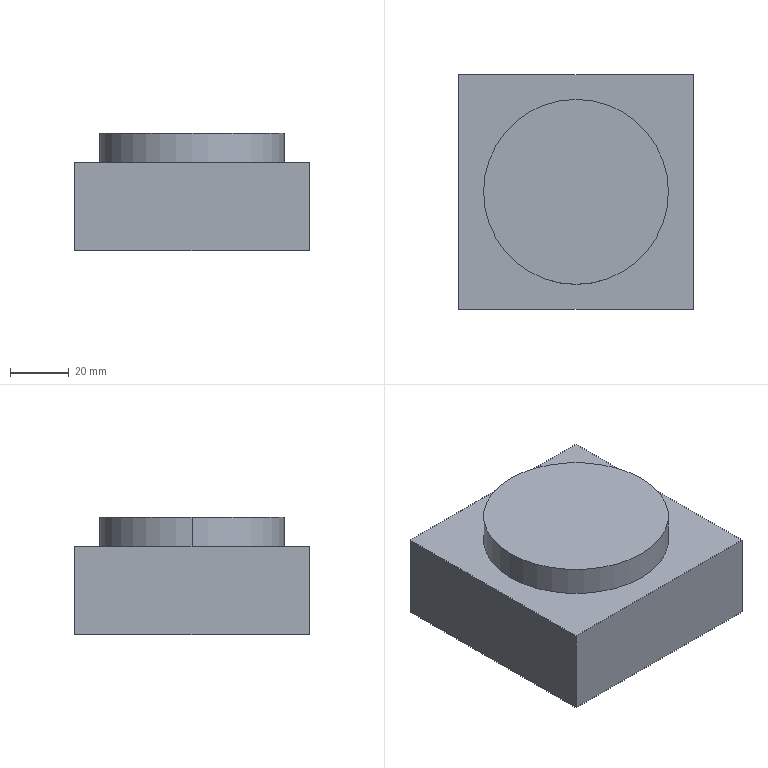Part | SolidWorks | features Extrusion 1, ICE 1 | 1 solid | 9 faces | box 80 x 80 x 40 mm | volume 223172 mm3 | plane 7 | cylinder 2 | commonest cylinder face diameters 63 x2
STEP:
#1=CARTESIAN_POINT('',(31.5,0.,40.));
#2=VERTEX_POINT('',#1);
#3=CARTESIAN_POINT('',(-31.5,0.,40.));
#4=VERTEX_POINT('',#3);
#5=CARTESIAN_POINT('',(0.,0.,40.));
#6=DIRECTION('',(0.,0.,1.));
#7=DIRECTION('',(1.,0.,0.));
#8=AXIS2_PLACEMENT_3D('',#5,#6,#7);
#9=CIRCLE('',#8,31.5);
#10=EDGE_CURVE('',#2,#4,#9,.T.);
#11=ORIENTED_EDGE('',*,*,#10,.F.);
#12=CARTESIAN_POINT('',(31.5,0.,30.));
#13=VERTEX_POINT('',#12);
#14=CARTESIAN_POINT('',(31.5,0.,40.));
#15=DIRECTION('',(0.,0.,-1.));
#16=VECTOR('',#15,1000.);
#17=LINE('',#14,#16);
#18=EDGE_CURVE('',#2,#13,#17,.T.);
#19=ORIENTED_EDGE('',*,*,#18,.T.);
#20=CARTESIAN_POINT('',(-31.5,0.,30.));
#21=VERTEX_POINT('',#20);
#22=CARTESIAN_POINT('',(0.,0.,30.));
#23=DIRECTION('',(0.,0.,1.));
#24=DIRECTION('',(1.,0.,0.));
#25=AXIS2_PLACEMENT_3D('',#22,#23,#24);
#26=CIRCLE('',#25,31.5);
#27=EDGE_CURVE('',#13,#21,#26,.T.);
#28=ORIENTED_EDGE('',*,*,#27,.T.);
#29=CARTESIAN_POINT('',(-31.5,0.,40.));
#30=DIRECTION('',(0.,0.,-1.));
#31=VECTOR('',#30,1000.);
#32=LINE('',#29,#31);
#33=EDGE_CURVE('',#4,#21,#32,.T.);
#34=ORIENTED_EDGE('',*,*,#33,.F.);
#35=EDGE_LOOP('',(#11,#19,#28,#34));
#36=FACE_OUTER_BOUND('',#35,.T.);
#37=CARTESIAN_POINT('',(0.,0.,40.));
#38=DIRECTION('',(0.,0.,-1.));
#39=DIRECTION('',(-1.,0.,0.));
#40=AXIS2_PLACEMENT_3D('',#37,#38,#39);
#41=CYLINDRICAL_SURFACE('',#40,31.5);
#42=ADVANCED_FACE('',(#36),#41,.T.);
#43=CARTESIAN_POINT('',(40.,-40.,0.));
#44=VERTEX_POINT('',#43);
#45=CARTESIAN_POINT('',(40.,40.,0.));
#46=VERTEX_POINT('',#45);
#47=CARTESIAN_POINT('',(40.,-40.,0.));
#48=DIRECTION('',(0.,1.,0.));
#49=VECTOR('',#48,1000.);
#50=LINE('',#47,#49);
#51=EDGE_CURVE('',#44,#46,#50,.T.);
#52=ORIENTED_EDGE('',*,*,#51,.T.);
#53=CARTESIAN_POINT('',(40.,40.,30.));
#54=VERTEX_POINT('',#53);
#55=CARTESIAN_POINT('',(40.,40.,30.));
#56=DIRECTION('',(0.,0.,-1.));
#57=VECTOR('',#56,1000.);
#58=LINE('',#55,#57);
#59=EDGE_CURVE('',#54,#46,#58,.T.);
#60=ORIENTED_EDGE('',*,*,#59,.F.);
#61=CARTESIAN_POINT('',(40.,-40.,30.));
#62=VERTEX_POINT('',#61);
#63=CARTESIAN_POINT('',(40.,-40.,30.));
#64=DIRECTION('',(0.,1.,0.));
#65=VECTOR('',#64,1000.);
#66=LINE('',#63,#65);
#67=EDGE_CURVE('',#62,#54,#66,.T.);
#68=ORIENTED_EDGE('',*,*,#67,.F.);
#69=CARTESIAN_POINT('',(40.,-40.,30.));
#70=DIRECTION('',(0.,0.,-1.));
#71=VECTOR('',#70,1000.);
#72=LINE('',#69,#71);
#73=EDGE_CURVE('',#62,#44,#72,.T.);
#74=ORIENTED_EDGE('',*,*,#73,.T.);
#75=EDGE_LOOP('',(#52,#60,#68,#74));
#76=FACE_OUTER_BOUND('',#75,.T.);
#77=CARTESIAN_POINT('',(40.,-40.,30.));
#78=DIRECTION('',(-1.,0.,0.));
#79=DIRECTION('',(0.,0.,1.));
#80=AXIS2_PLACEMENT_3D('',#77,#78,#79);
#81=PLANE('',#80);
#82=ADVANCED_FACE('',(#76),#81,.F.);
#83=CARTESIAN_POINT('',(-40.,40.,0.));
#84=VERTEX_POINT('',#83);
#85=CARTESIAN_POINT('',(-40.,40.,0.));
#86=DIRECTION('',(-1.,0.,0.));
#87=VECTOR('',#86,1000.);
#88=LINE('',#85,#87);
#89=EDGE_CURVE('',#46,#84,#88,.T.);
#90=ORIENTED_EDGE('',*,*,#89,.T.);
#91=CARTESIAN_POINT('',(-40.,40.,30.));
#92=VERTEX_POINT('',#91);
#93=CARTESIAN_POINT('',(-40.,40.,30.));
#94=DIRECTION('',(0.,0.,-1.));
#95=VECTOR('',#94,1000.);
#96=LINE('',#93,#95);
#97=EDGE_CURVE('',#92,#84,#96,.T.);
#98=ORIENTED_EDGE('',*,*,#97,.F.);
#99=CARTESIAN_POINT('',(-40.,40.,30.));
#100=DIRECTION('',(-1.,0.,0.));
#101=VECTOR('',#100,1000.);
#102=LINE('',#99,#101);
#103=EDGE_CURVE('',#54,#92,#102,.T.);
#104=ORIENTED_EDGE('',*,*,#103,.F.);
#105=ORIENTED_EDGE('',*,*,#59,.T.);
#106=EDGE_LOOP('',(#90,#98,#104,#105));
#107=FACE_OUTER_BOUND('',#106,.T.);
#108=CARTESIAN_POINT('',(-40.,40.,30.));
#109=DIRECTION('',(0.,-1.,0.));
#110=DIRECTION('',(0.,0.,-1.));
#111=AXIS2_PLACEMENT_3D('',#108,#109,#110);
#112=PLANE('',#111);
#113=ADVANCED_FACE('',(#107),#112,.F.);
#114=CARTESIAN_POINT('',(-40.,-40.,0.));
#115=VERTEX_POINT('',#114);
#116=CARTESIAN_POINT('',(-40.,-40.,0.));
#117=DIRECTION('',(0.,-1.,0.));
#118=VECTOR('',#117,1000.);
#119=LINE('',#116,#118);
#120=EDGE_CURVE('',#84,#115,#119,.T.);
#121=ORIENTED_EDGE('',*,*,#120,.T.);
#122=CARTESIAN_POINT('',(-40.,-40.,30.));
#123=VERTEX_POINT('',#122);
#124=CARTESIAN_POINT('',(-40.,-40.,30.));
#125=DIRECTION('',(0.,0.,-1.));
#126=VECTOR('',#125,1000.);
#127=LINE('',#124,#126);
#128=EDGE_CURVE('',#123,#115,#127,.T.);
#129=ORIENTED_EDGE('',*,*,#128,.F.);
#130=CARTESIAN_POINT('',(-40.,-40.,30.));
#131=DIRECTION('',(0.,-1.,0.));
#132=VECTOR('',#131,1000.);
#133=LINE('',#130,#132);
#134=EDGE_CURVE('',#92,#123,#133,.T.);
#135=ORIENTED_EDGE('',*,*,#134,.F.);
#136=ORIENTED_EDGE('',*,*,#97,.T.);
#137=EDGE_LOOP('',(#121,#129,#135,#136));
#138=FACE_OUTER_BOUND('',#137,.T.);
#139=CARTESIAN_POINT('',(-40.,-40.,30.));
#140=DIRECTION('',(1.,0.,0.));
#141=DIRECTION('',(0.,0.,-1.));
#142=AXIS2_PLACEMENT_3D('',#139,#140,#141);
#143=PLANE('',#142);
#144=ADVANCED_FACE('',(#138),#143,.F.);
#145=CARTESIAN_POINT('',(-40.,-40.,0.));
#146=DIRECTION('',(1.,0.,0.));
#147=VECTOR('',#146,1000.);
#148=LINE('',#145,#147);
#149=EDGE_CURVE('',#115,#44,#148,.T.);
#150=ORIENTED_EDGE('',*,*,#149,.T.);
#151=ORIENTED_EDGE('',*,*,#73,.F.);
#152=CARTESIAN_POINT('',(-40.,-40.,30.));
#153=DIRECTION('',(1.,0.,0.));
#154=VECTOR('',#153,1000.);
#155=LINE('',#152,#154);
#156=EDGE_CURVE('',#123,#62,#155,.T.);
#157=ORIENTED_EDGE('',*,*,#156,.F.);
#158=ORIENTED_EDGE('',*,*,#128,.T.);
#159=EDGE_LOOP('',(#150,#151,#157,#158));
#160=FACE_OUTER_BOUND('',#159,.T.);
#161=CARTESIAN_POINT('',(-40.,-40.,30.));
#162=DIRECTION('',(0.,1.,0.));
#163=DIRECTION('',(0.,0.,1.));
#164=AXIS2_PLACEMENT_3D('',#161,#162,#163);
#165=PLANE('',#164);
#166=ADVANCED_FACE('',(#160),#165,.F.);
#167=CARTESIAN_POINT('',(0.,0.,30.));
#168=DIRECTION('',(0.,0.,1.));
#169=DIRECTION('',(1.,0.,0.));
#170=AXIS2_PLACEMENT_3D('',#167,#168,#169);
#171=CIRCLE('',#170,31.5);
#172=EDGE_CURVE('',#21,#13,#171,.T.);
#173=ORIENTED_EDGE('',*,*,#172,.F.);
#174=ORIENTED_EDGE('',*,*,#27,.F.);
#175=EDGE_LOOP('',(#173,#174));
#176=FACE_BOUND('',#175,.T.);
#177=ORIENTED_EDGE('',*,*,#67,.T.);
#178=ORIENTED_EDGE('',*,*,#103,.T.);
#179=ORIENTED_EDGE('',*,*,#134,.T.);
#180=ORIENTED_EDGE('',*,*,#156,.T.);
#181=EDGE_LOOP('',(#177,#178,#179,#180));
#182=FACE_OUTER_BOUND('',#181,.T.);
#183=CARTESIAN_POINT('',(0.,0.,30.));
#184=DIRECTION('',(0.,0.,-1.));
#185=DIRECTION('',(-1.,0.,0.));
#186=AXIS2_PLACEMENT_3D('',#183,#184,#185);
#187=PLANE('',#186);
#188=ADVANCED_FACE('',(#176,#182),#187,.F.);
#189=ORIENTED_EDGE('',*,*,#51,.F.);
#190=ORIENTED_EDGE('',*,*,#149,.F.);
#191=ORIENTED_EDGE('',*,*,#120,.F.);
#192=ORIENTED_EDGE('',*,*,#89,.F.);
#193=EDGE_LOOP('',(#189,#190,#191,#192));
#194=FACE_OUTER_BOUND('',#193,.T.);
#195=CARTESIAN_POINT('',(0.,0.,0.));
#196=DIRECTION('',(0.,0.,-1.));
#197=DIRECTION('',(-1.,0.,0.));
#198=AXIS2_PLACEMENT_3D('',#195,#196,#197);
#199=PLANE('',#198);
#200=ADVANCED_FACE('',(#194),#199,.T.);
#201=ORIENTED_EDGE('',*,*,#18,.F.);
#202=CARTESIAN_POINT('',(0.,0.,40.));
#203=DIRECTION('',(0.,0.,1.));
#204=DIRECTION('',(1.,0.,0.));
#205=AXIS2_PLACEMENT_3D('',#202,#203,#204);
#206=CIRCLE('',#205,31.5);
#207=EDGE_CURVE('',#4,#2,#206,.T.);
#208=ORIENTED_EDGE('',*,*,#207,.F.);
#209=ORIENTED_EDGE('',*,*,#33,.T.);
#210=ORIENTED_EDGE('',*,*,#172,.T.);
#211=EDGE_LOOP('',(#201,#208,#209,#210));
#212=FACE_OUTER_BOUND('',#211,.T.);
#213=CARTESIAN_POINT('',(0.,0.,40.));
#214=DIRECTION('',(0.,0.,-1.));
#215=DIRECTION('',(-1.,0.,0.));
#216=AXIS2_PLACEMENT_3D('',#213,#214,#215);
#217=CYLINDRICAL_SURFACE('',#216,31.5);
#218=ADVANCED_FACE('',(#212),#217,.T.);
#219=ORIENTED_EDGE('',*,*,#207,.T.);
#220=ORIENTED_EDGE('',*,*,#10,.T.);
#221=EDGE_LOOP('',(#219,#220));
#222=FACE_OUTER_BOUND('',#221,.T.);
#223=CARTESIAN_POINT('',(0.,0.,40.));
#224=DIRECTION('',(0.,0.,1.));
#225=DIRECTION('',(1.,0.,0.));
#226=AXIS2_PLACEMENT_3D('',#223,#224,#225);
#227=PLANE('',#226);
#228=ADVANCED_FACE('',(#222),#227,.T.);
#229=CLOSED_SHELL('',(#42,#82,#113,#144,#166,#188,#200,#218,#228));
#230=MANIFOLD_SOLID_BREP('',#229);
#231=CARTESIAN_POINT('',(0.,0.,0.));
#232=DIRECTION('',(0.,0.,1.));
#233=DIRECTION('',(1.,0.,0.));
#234=AXIS2_PLACEMENT_3D('',#231,#232,#233);
#235=(LENGTH_UNIT()NAMED_UNIT(*)SI_UNIT(.MILLI.,.METRE.));
#236=UNCERTAINTY_MEASURE_WITH_UNIT(LENGTH_MEASURE(0.00001),#235,'','');
#237=(NAMED_UNIT(*)PLANE_ANGLE_UNIT()SI_UNIT($,.RADIAN.));
#238=(NAMED_UNIT(*)SI_UNIT($,.STERADIAN.)SOLID_ANGLE_UNIT());
#239=(GEOMETRIC_REPRESENTATION_CONTEXT(3)GLOBAL_UNCERTAINTY_ASSIGNED_CONTEXT((#236))GLOBAL_UNIT_ASSIGNED_CONTEXT((#235,#237,#238))REPRESENTATION_CONTEXT('',''));
#240=ADVANCED_BREP_SHAPE_REPRESENTATION('',(#230,#234),#239);